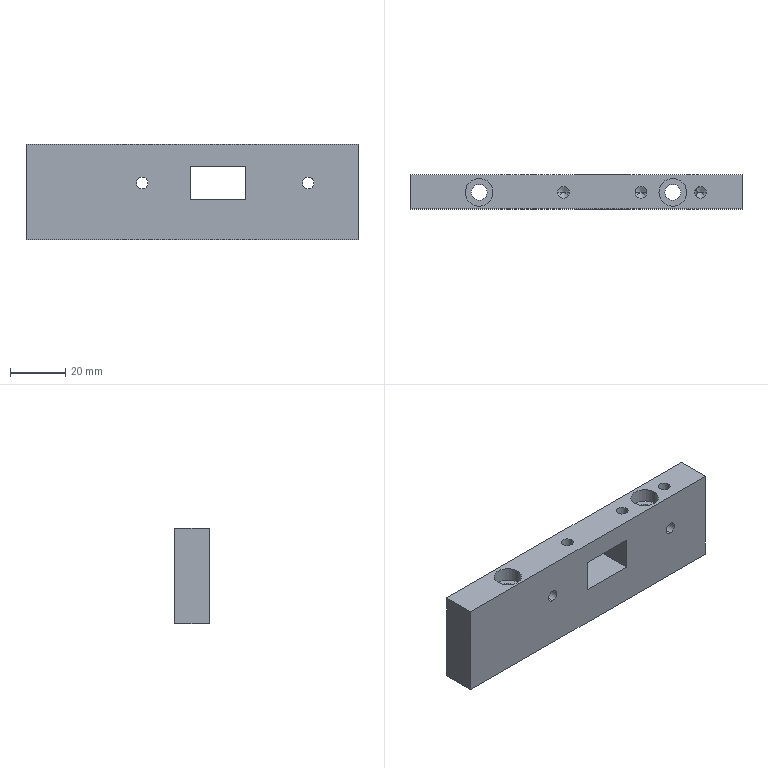Part | STEP file | magnetizing side block | 1 solid | 36 faces | box 120 x 12.3 x 34.5 mm | volume 44752 mm3 | cylinder 18 | plane 12 | cone 6 | commonest cylinder face diameters 4.2 x10 5.8 x4 10 x4